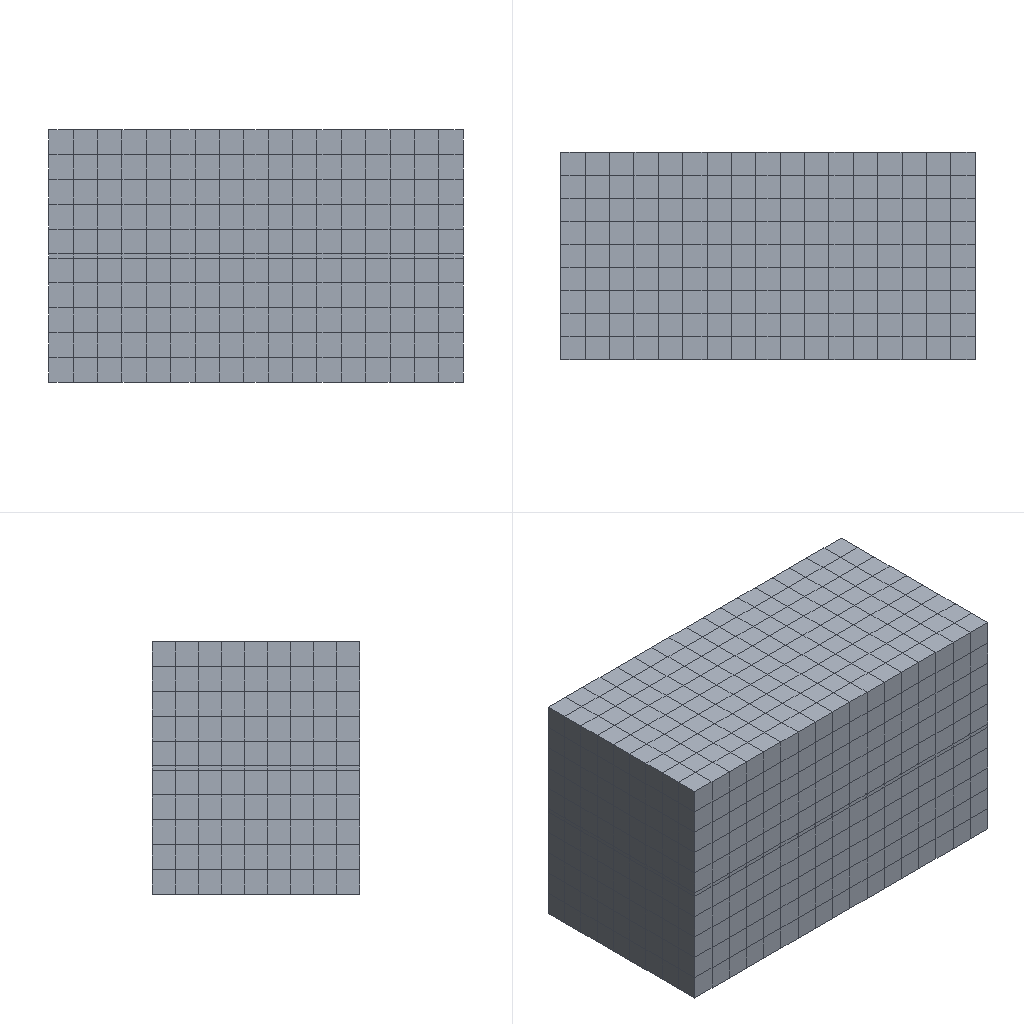Simulation study | ansys workbench
Ansys APDL input file, long lists of numbers shortened:
/batch
/config,noeldb,1     ! force off writing results to database
*get,_wallstrt,active,,time,wall
! ANSYS input file written by Workbench version 2022 R2
! File used for geometry attach:
/title,wbnew--__ (B5)
! ****** Begin Custom Load Command Snippet ******
/COM, ACT Extensions:
/COM,     LSDYNA, 2022.2
/COM,/COM,     ANSYSMotion, 2022.2
/COM,
! ****** End   Custom Load Command Snippet ******
*DIM,_wb_ProjectScratch_dir,string,248
_wb_ProjectScratch_dir(1) = ''
*DIM,_wb_SolverFiles_dir,string,248
_wb_SolverFiles_dir(1) = ''
*DIM,_wb_userfiles_dir,string,248
_wb_userfiles_dir(1) = ''
/com,--- Data in consistent NMM units. See Solving Units in the help system for more information.
/units,MPA
/nopr
/wb,file,start              !  signify a WB generated input file
/prep7
! Turn off shape checking because checks already performed inside WB mesher.
! See help system for more information.
SHPP,OFF,,NOWARN
/nolist
etcon,set             ! allow ANSYS to choose best KEYOP's for 180x elements, resets any applicable keyopt to MAPDL defaults
/com,*********** Nodes for the whole assembly ***********
nblock,3,,10062
(1i9,3e20.9e3)
     7945     4.411764706E+00     1.944444444E+00     3.000000000E+00
! (9147 more lines like these left out)
-1
/wb,elem,start            !  set before creation of elements
/com,*********** Elements for Body 1 "__" ***********
et,1,186
keyo,1,2,1          ! set full integration on SOLID186
eblock,19,solid,,765
(19i9)
        1        1        1        1        0        0        0        0       20        0        1        1     1001      862      824      640     1080      861      853
! (1529 more lines like these left out)
-1
/com,*********** Elements for Body 2 "__" ***********
et,2,186
keyo,2,2,1          ! set full integration on SOLID186
eblock,19,solid,,765
(19i9)
        2        2        2        2        0        0        0        0       20        0      766     3973     4793     4874     5041     4612     4872     4873     5045
! (1529 more lines like these left out)
-1
/com,*********** Elements for Body 3 "__" ***********
et,3,186
keyo,3,2,1          ! set full integration on SOLID186
eblock,19,solid,,153
(19i9)
        3        3        3        3        0        0        0        0       20        0     1531     8072     8297     8269     8268     8073     8208     8235     8236
! (305 more lines like these left out)
-1
/wb,elem,end               !  done creating elements
/com,*********** Send User Defined Coordinate System(s) ***********
csys,0
toffst,273.15,  ! Temperature offset from absolute zero
/com,*********** Set Reference Temperature ***********
tref,22.
/wb,mat,start              !  starting to send materials
/com,*********** Send Materials ***********
MP,DENS,1,3.2e-09,	! tonne mm^-3
MP,ALPX,1,3.5e-06,	! C^-1
MP,KXX,1,20,	! tonne mm s^-3 C^-1
MP,C,1,750000000,	! mm^2 s^-2 C^-1
MP,EX,1,300000,	! tonne s^-2 mm^-1
MP,NUXY,1,0.27,
Temperature = 'TEMP' ! Temperature
MP,DENS,2,4.51e-09,	! tonne mm^-3
MP,CTEX,2,9e-06,	! C^-1
MP,C,2,530000000,	! mm^2 s^-2 C^-1
MP,KXX,2,19,	! tonne mm s^-3 C^-1
MP,RSVX,2,0.0017,	! ohm mm
MP,EX,2,110000,	! tonne s^-2 mm^-1
MP,NUXY,2,0.34,
MP,MURX,2,1,
MP,DENS,3,9.8e-09,	! tonne mm^-3
MP,CTEX,3,1.9e-05,	! C^-1
MP,EX,3,75000,	! tonne s^-2 mm^-1
MP,NUXY,3,0.35,
MP,KXX,3,110,	! tonne mm s^-3 C^-1
MP,C,3,420000000,	! mm^2 s^-2 C^-1
/wb,mat,end                !  done sending materials
!************************* Model Summary ********************
!__,	SI3N4,	matid,	1
!__,	钛合金,	matid,	2
!__,	AG-CU-TI,	matid,	3
!************************* End Model Summary ********************
! get the diagonal of the bounding box. Needed later for other things
*get,_xmin,node,,mnloc,x
*get,_ymin,node,,mnloc,y
*get,_zmin,node,,mnloc,z
*get,_xmax,node,,mxloc,x
*get,_ymax,node,,mxloc,y
*get,_zmax,node,,mxloc,z
_ASMDIAG=(_xmax-_xmin)*(_xmax-_xmin)+(_ymax-_ymin)*(_ymax-_ymin)+(_zmax-_zmin)*(_zmax-_zmin)
_ASMDIAG=SQRT(_ASMDIAG)
/wb,contact,start          !  starting to send contact
/com,*********** Create Contact "接触区域" ***********
/com,            Real Constant Set For Above Contact Is 5 & 4
*set,tid,5
*set,cid,4
r,tid
r,cid
et,tid,170
et,cid,174
eblock,10,,,153
(15i9)
     3174        5        5        5        0      853      640     1080      861     3119     3120     3583     3574
! (152 more lines like these left out)
-1
eblock,10,,,153
(15i9)
     3327        4        4        4        0      853      640     1080      861     3119     3120     3583     3574
! (152 more lines like these left out)
-1
eblock,10,,,153
(15i9)
     3480        4        5        4        0     8236     8073     8208     8235     8716     8715     9008     9062
! (152 more lines like these left out)
-1
eblock,10,,,153
(15i9)
     3633        5        4        5        0     8236     8073     8208     8235     8716     8715     9008     9062
! (152 more lines like these left out)
-1
keyo,cid,8,2               ! auto create asymmetric contact (from Program Controlled setting)
keyo,cid,10,0              ! adjust contact stiffness each NR iteration (from Program Controlled setting)
keyo,cid,12,5              ! bonded always
keyo,cid,18,1              ! small sliding turned on by application
keyo,cid,2,0               ! augmented Lagrange (from Program Controlled setting)
keyo,cid,4,0               ! on Gauss point (from Program Controlled setting)
keyo,cid,9,1               ! ignore initial gaps/penetration
keyo,cid,7,0               ! No Prediction
rmod,tid,3,10.      ! FKN
rmod,tid,5,0.       ! ICONT
rmod,tid,6,0.       ! PINB
rmod,tid,10,0.      ! CNOF
rmod,tid,12,0.      ! FKT
rmod,tid,36,34      ! WB DSID
rmod,cid,3,10.      ! FKN
rmod,cid,5,0.       ! ICONT
rmod,cid,6,0.       ! PINB
rmod,cid,10,0.      ! CNOF
rmod,cid,12,0.      ! FKT
rmod,cid,36,34      ! WB DSID
/com,*********** Create Contact "接触区域 2" ***********
/com,            Real Constant Set For Above Contact Is 7 & 6
*set,tid,7
*set,cid,6
r,tid
r,cid
et,tid,170
et,cid,174
eblock,10,,,153
(15i9)
     3786        7        7        7        0     4776     4613     4748     4775     7096     7095     7388     7442
! (152 more lines like these left out)
-1
eblock,10,,,153
(15i9)
     3939        6        6        6        0     4776     4613     4748     4775     7096     7095     7388     7442
! (152 more lines like these left out)
-1
eblock,10,,,153
(15i9)
     4092        6        7        6        0     8297     8072     8268     8269     8712     8711     9113     9114
! (152 more lines like these left out)
-1
eblock,10,,,153
(15i9)
     4245        7        6        7        0     8297     8072     8268     8269     8712     8711     9113     9114
! (152 more lines like these left out)
-1
keyo,cid,8,2               ! auto create asymmetric contact (from Program Controlled setting)
keyo,cid,10,0              ! adjust contact stiffness each NR iteration (from Program Controlled setting)
keyo,cid,12,5              ! bonded always
keyo,cid,18,1              ! small sliding turned on by application
keyo,cid,2,0               ! augmented Lagrange (from Program Controlled setting)
keyo,cid,4,0               ! on Gauss point (from Program Controlled setting)
keyo,cid,9,1               ! ignore initial gaps/penetration
keyo,cid,7,0               ! No Prediction
rmod,tid,3,10.      ! FKN
rmod,tid,5,0.       ! ICONT
rmod,tid,6,0.       ! PINB
rmod,tid,10,0.      ! CNOF
rmod,tid,12,0.      ! FKT
rmod,tid,36,37      ! WB DSID
rmod,cid,3,10.      ! FKN
rmod,cid,5,0.       ! ICONT
rmod,cid,6,0.       ! PINB
rmod,cid,10,0.      ! CNOF
rmod,cid,12,0.      ! FKT
rmod,cid,36,37      ! WB DSID
nsel,all
esel,all
/wb,contact,end            !  done creating contacts
/golist
/wb,load,start             !  starting to send loads
/com,********* Frictionless Supports Y *********
CMBLOCK,_FRICSUY,NODE,      688
(8i10)
       794       795       796       797       798       799       800       801
! (85 more lines like these left out)
cmsel,s,_FRICSUY
d,all,uy,0
nsel,all
/com,******* Constant Zero Displacement X *******
CMBLOCK,_DISPZEROUX,NODE,       76
(8i10)
       785       786       787       788       789       790       791       792
! (9 more lines like these left out)
cmsel,s,_DISPZEROUX
d,all,ux,0
nsel,all
/com,******* Constant Zero Displacement Y *******
CMBLOCK,_DISPZEROUY,NODE,       72
(8i10)
       785       786       787       788       789       790       791       792
! (8 more lines like these left out)
cmsel,s,_DISPZEROUY
d,all,uy,0
nsel,all
/com,******* Constant Zero Displacement Z *******
CMBLOCK,_DISPZEROUZ,NODE,       76
(8i10)
       785       786       787       788       789       790       791       792
! (9 more lines like these left out)
cmsel,s,_DISPZEROUZ
d,all,uz,0
nsel,all
/com,*********** Create Load Variation Table for Imported Load "________" ***********
*DIM, _lv_54__0, TABLE, 31, 9148, 1, TIME, NODE, ,
*PREAD, _lv_54__0, 292768
  0.000000000000e+00  1.000000000000e-02  1.000003333333e-02  1.333333333000e-02
  1.333336666333e-02  1.666666666000e-02  1.666676666000e-02  2.666666665000e-02
! (73190 more lines like these left out)
END PREAD
CMBLOCK,_LV_54__SELECTION,NODE,     9148
(8i10)
         1         2         3         4         5         6         7         8
! (1143 more lines like these left out)
/gst,on,on
fini
*get,_numnode,node,0,count
*get,_numelem,elem,0,count
*get, _MAXELEMNUM, elem, 0, NUM, MAX
*get, _MAXNODENUM, node, 0, NUM, MAX
*get, _MAXELEMTYPE, etyp, 0, NUM, MAX
*get, _MAXREALCONST, rcon, 0, NUM, MAX
/go
/wb,load,end               !  done creating loads
/com,--- Number of total nodes = %_numnode%
/com,--- Number of contact elements = 1224
/com,--- Number of spring elements = 0
/com,--- Number of bearing elements = 0
/com,--- Number of solid elements = 1683
/com,--- Number of condensed parts = 0
/com,--- Number of total elements = %_numelem%
*get,_wallbsol,active,,time,wall
/com,****************************************************************************
/com,*************************    SOLUTION       ********************************
/com,****************************************************************************
/solu
antype,4                   ! transient analysis
nlgeom,on                  ! Turn on Large Deformation Effects
kbc,1                      ! stepped BC's
_thickRatio=0.667   ! Ratio of thick parts in the model
eqsl,pcg,1e-8,,,,,,1
cntr,print,1               ! print out contact info and also make no initial contact an error
dmpoption,emat,no             ! Don't combine emat file for DANSYS
dmpoption,esav,no             ! Don't combine esav file for DANSYS
trnopt,full,,,,,hht        ! HHT time integration method
tintp, mosp			! Choose transient integration settings for moderate speed application
nldiag,cont,iter           ! print out contact info each equilibrium iteration
rescontrol,define,last,last,,dele	   ! Program Controlled
/com,****************************************************
/com,******************* SOLVE FOR LS 1 OF 1 ****************
/nopr
/com,*********** Create Imported Load "________" ***********
/nopr
bf,_lv_54__selection,temp,%_lv_54__0%
/gopr
/gopr
autots,on                   ! User turned on automatic time stepping
deltim,0.01,0.001,0.1,OFF
time,1.
timint,on                  ! Turn on time integration effects
outres,erase
outres,all,none
outres,nsol,all,
outres,rsol,all
outres,eangl,all
outres,etmp,all
outres,veng,all
outres,strs,all,
outres,epel,all,
outres,eppl,all,
outres,epth,all,
outres,cont,all,
outres,v,all,
outres,a,all,
! *********** WB SOLVE COMMAND ***********
! check interactive state
*get,ANSINTER_,active,,int
*if,ANSINTER_,ne,0,then
/eof
*endif
solve
/com *************** Write FE CONNECTORS *********
CEWRITE,file,ce,,INTE
/com,****************************************************
/com,*************** FINISHED SOLVE FOR LS 1 *************
*get,_wallasol,active,,time,wall
/nopr
*get,_numnode,node,0,count
*get,_numelem,elem,0,count
*get, _MAXELEMNUM, elem, 0, NUM, MAX
*get, _MAXNODENUM, node, 0, NUM, MAX,,,INTERNAL
*get, _MAXELEMTYPE, etyp, 0, NUM, MAX
*get, _MAXREALCONST, rcon, 0, NUM, MAX
*get,_NSOLTHREADS,active,0,ntfs
*get,_NSOLPROCESSES,active,0,npfs
/gopr
*get,_PCGITER,active,,solu,cgiter
/post1
/com,*********** Deleting tables created for Imported Loads ***********
_lv_54__0=
xmlo,ENCODING,ISO-8859-1
xmlo,parm
/xml,parm,xml
fini
/gopr
*get,_walldone,active,,time,wall
_preptime=(_wallbsol-_wallstrt)*3600
_solvtime=(_wallasol-_wallbsol)*3600
_posttime=(_walldone-_wallasol)*3600
_totaltim=(_walldone-_wallstrt)*3600
*get,_dlbratio,active,0,solu,dlbr
*get,_combtime,active,0,solu,comb
*get,_ssmode,active,0,solu,ssmm
*get,_ndofs,active,0,solu,ndof
*get,_sol_end_time,active,0,set,time
*if,_sol_end_time,eq,1.,then
/fclean				!clean distributed files
*endif
/com,--- Total number of nodes = %_numnode%
/com,--- Total number of elements = %_numelem%
/com,--- Element load balance ratio = %_dlbratio%
/com,--- Time to combine distributed files = %_combtime%
/com,--- Sparse memory mode = %_ssmode%
/com,--- Number of DOF = %_ndofs%
/wb,file,end               ! done with WB generated input